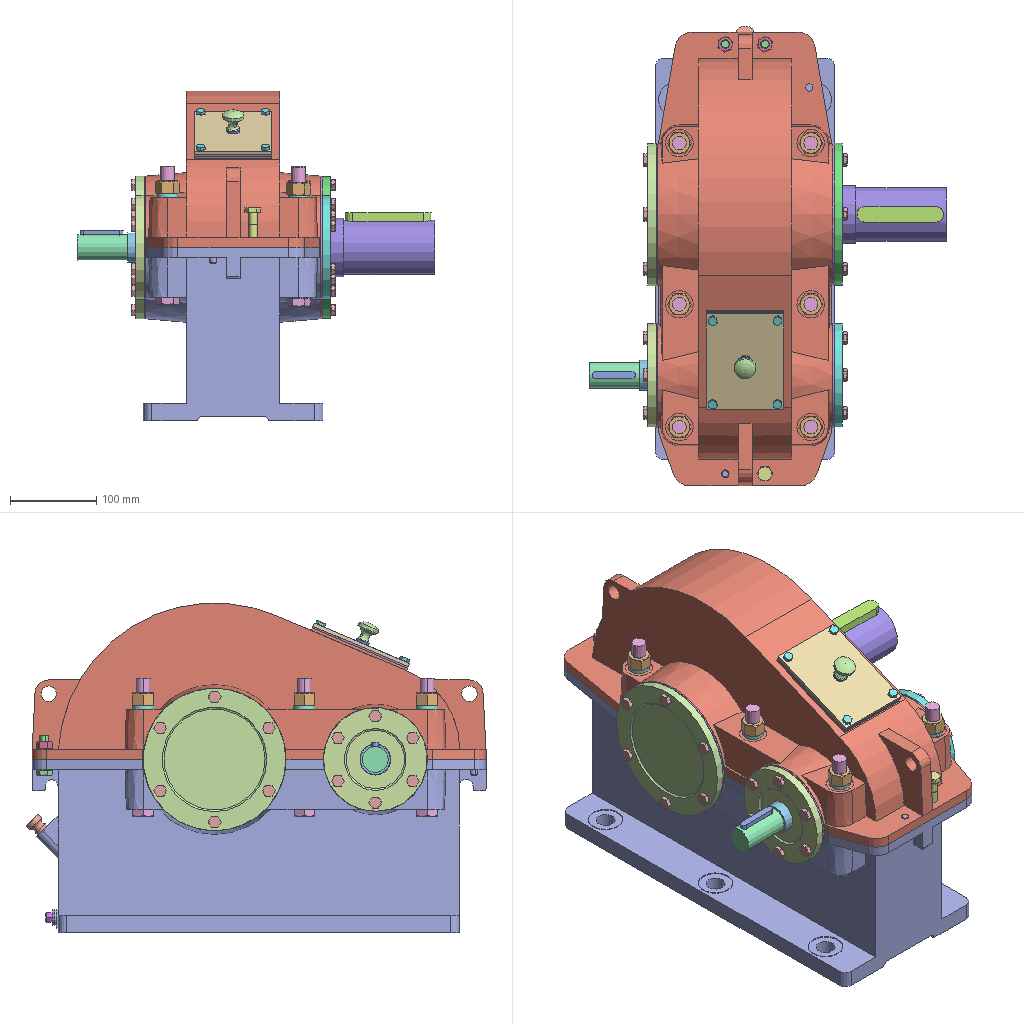Assembly | NX | 39 different items | 95 placed | box 413 x 532 x 381 mm
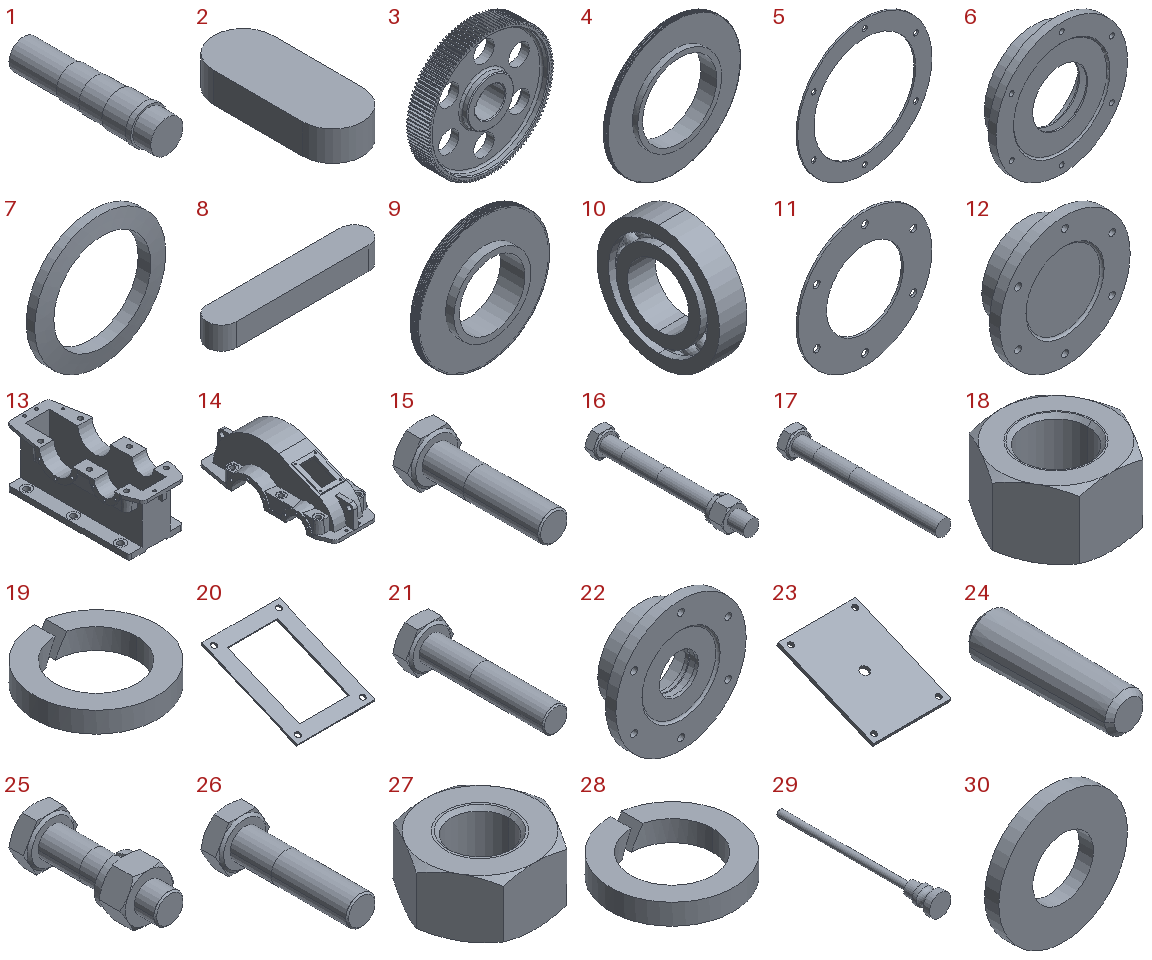Parts list (item | quantity | parent item | size | volume | features):
1 | x1 | - | 79 x 311 x 79 mm | 1137641 mm3 | features DATUM_CSYS 9, EXTRUDE 8, SKETCH 8, BLEND 2
2 | x1 | - | 20 x 50 x 10 mm | 9142 mm3 | features DATUM_CSYS 2, EXTRUDE 1, SKETCH 1
3 | x1 | - | 322.473 x 55 x 322.494 mm | 1796167 mm3 | features BREP 127, META 127, DATUM_CSYS 10, SKETCH 9, EXTRACT_DATUM_AXIS 8, HOLE PACKAGE 7, SIMPLE HOLE 7, EXTRACT_FACE 6, Instance Feature 6, EXTRUDE 3, EXTRACT_DATUM_PLANE 2, BLEND 1, CHAMFER 1, CYLINDER 1, FSET 1, Mirror Feature 1, Pattern Feature 1
4 | x2 | - | 125 x 15 x 125 mm | 52069 mm3 | features DATUM_CSYS 4, SKETCH 3, EXTRUDE 2, HOLE PACKAGE 1, SIMPLE HOLE 1, SWP104 1
5 | x2 | - | 165 x 2 x 165 mm | 17882 mm3 | features DATUM_CSYS 12, SKETCH 11, HOLE PACKAGE 9, SIMPLE HOLE 9, EXTRACT_DATUM_AXIS 6, EXTRACT_FACE 6, Instance Feature 5, EXTRUDE 4, BLEND 2, DELETE FACE 1, OFFSET_REGION 1, Pattern Feature 1, SWP104 1
6 | x1 | - | 165 x 34.6 x 165 mm | 207010 mm3 | features DATUM_CSYS 10, HOLE PACKAGE 9, SIMPLE HOLE 9, SKETCH 9, EXTRACT_DATUM_AXIS 6, EXTRACT_FACE 6, Instance Feature 5, BLEND 2, EXTRUDE 2, Pattern Feature 1, SWP104 1
7 | x1 | - | 93.171 x 8.968 x 93.171 mm | 22814 mm3 | features DATUM_CSYS 3, SKETCH 2, EXTRUDE 1, SWP104 1
8 | x1 | - | 100 x 18 x 14 mm | 24227 mm3 | features DATUM_CSYS 2, BLEND 1, EXTRUDE 1, SKETCH 1
9 | x2 | - | 80 x 15 x 80 mm | 23126 mm3 | features DATUM_CSYS 5, SKETCH 4, EXTRUDE 3, SWP104 1
10 | x2 | - | 18 x 80 x 80 mm | 52959 mm3 | features BREP 17
11 | x2 | - | 120 x 2 x 120 mm | 14781 mm3 | features DATUM_CSYS 12, SKETCH 11, HOLE PACKAGE 9, SIMPLE HOLE 9, EXTRACT_DATUM_AXIS 6, EXTRACT_FACE 6, Instance Feature 5, EXTRUDE 4, BLEND 2, DELETE FACE 1, Pattern Feature 1, REPLACE_FACE 1, SWP104 1
12 | x1 | - | 120 x 36.6 x 120 mm | 144277 mm3 | features DATUM_CSYS 9, HOLE PACKAGE 9, SIMPLE HOLE 9, SKETCH 8, EXTRACT_DATUM_AXIS 6, EXTRACT_FACE 6, Instance Feature 5, BLEND 2, EXTRUDE 2, DELETE FACE 1, Pattern Feature 1
13 | x1 | - | 208 x 525 x 200.222 mm | 4335166 mm3 | features SIMPLE HOLE 56, DATUM_CSYS 27, HOLE PACKAGE 26, SKETCH 26, EXTRUDE 18, EXTRACT_FACE 16, EXTRACT_DATUM_AXIS 10, BLEND 8, CBORE_HOLE 7, EXTRACT_DATUM_PLANE 6, FSET 6, Instance Feature 5, Mirror Feature 5, DRAFT 4, EXTRACT_STRING 2
14 | x1 | - | 202 x 525 x 181 mm | 2847836 mm3 | features SIMPLE HOLE 56, DATUM_CSYS 27, HOLE PACKAGE 26, SKETCH 26, EXTRUDE 18, EXTRACT_FACE 16, EXTRACT_DATUM_AXIS 10, BLEND 8, CBORE_HOLE 7, EXTRACT_DATUM_PLANE 6, FSET 6, Instance Feature 5, Mirror Feature 5, DRAFT 4, EXTRACT_STRING 2
15 | x1 | - | 18.475 x 46.4 x 16 mm | 5258 mm3 | features BREP 2
16 | x6 | - | 27.713 x 160 x 24.4 mm | 46237 mm3 | features BREP 5, DELETE FACE 1, OFFSET_REGION 1
17 | x6 | in 16 | 27.713 x 160 x 24 mm | 38117 mm3 | features BREP 2, DELETE FACE 1, OFFSET_REGION 1
18 | x6 | in 16 | 27.713 x 24 x 14.8 mm | 7082 mm3 | features BREP 2
19 | x6 | in 16 | 24.4 x 24.4 x 4.1 mm | 1037 mm3 | features BREP 1
20 | x1 | - | 90 x 111.242 x 48.729 mm | 10934 mm3 | features SIMPLE HOLE 56, DATUM_CSYS 27, HOLE PACKAGE 26, SKETCH 26, EXTRUDE 18, EXTRACT_FACE 16, EXTRACT_DATUM_AXIS 10, BLEND 8, CBORE_HOLE 7, EXTRACT_DATUM_PLANE 6, FSET 6, Instance Feature 5, Mirror Feature 5, DRAFT 4, EXTRACT_STRING 2, OFFSET_REGION 1
21 | x4 | - | 11.547 x 34 x 10 mm | 1354 mm3 | features BREP 2
22 | x1 | - | 120 x 36.6 x 120 mm | 131277 mm3 | features DATUM_CSYS 10, HOLE PACKAGE 9, SIMPLE HOLE 9, SKETCH 9, EXTRACT_DATUM_AXIS 6, EXTRACT_FACE 6, Instance Feature 5, BLEND 2, EXTRUDE 2, Pattern Feature 1, SWP104 1
23 | x1 | - | 90 x 112.024 x 50.57 mm | 42433 mm3 | features SIMPLE HOLE 57, DATUM_CSYS 28, HOLE PACKAGE 27, SKETCH 27, EXTRUDE 18, EXTRACT_FACE 16, EXTRACT_DATUM_AXIS 10, BLEND 8, CBORE_HOLE 7, EXTRACT_DATUM_PLANE 6, FSET 6, Instance Feature 5, Mirror Feature 5, DRAFT 4, EXTRACT_STRING 2, DELETE FACE 1, OFFSET_REGION 1
24 | x1 | - | 8.911 x 30 x 8.911 mm | 1668 mm3 | features BREP 1
25 | x2 | - | 18.475 x 46.4 x 16 mm | 7344 mm3 | features BREP 5
26 | x2 | in 25 | 18.475 x 46.4 x 16 mm | 5258 mm3 | features BREP 2
27 | x2 | in 25 | 18.475 x 16 x 8.4 mm | 1823 mm3 | features BREP 2
28 | x2 | in 25 | 15.4 x 15.4 x 2.6 mm | 263.016 mm3 | features BREP 1
29 | x1 | - | 20 x 148 x 20 mm | 8375 mm3 | features DATUM_CSYS 6, SKETCH 5, EXTRUDE 4, SWP104 1
30 | x1 | - | 18 x 2 x 18 mm | 395.448 mm3 | features DATUM_CSYS 2, EXTRUDE 1, SKETCH 1
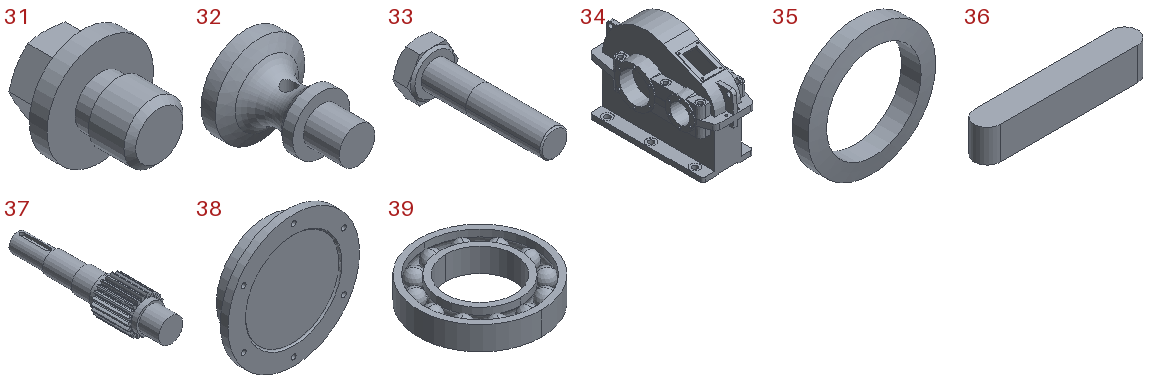31 | x1 | - | 18 x 20 x 18 mm | 2187 mm3 | features DATUM_CSYS 6, SKETCH 5, EXTRUDE 4, CHAMFER 1, SWP104 1
32 | x1 | - | 25 x 35 x 25 mm | 6314 mm3 | features DATUM_CSYS 5, SKETCH 4, EXTRUDE 3, SWP104 1
33 | x24 | - | 15.011 x 40.3 x 13 mm | 2901 mm3 | features BREP 2
34 | x1 | - | 208 x 525 x 381.222 mm | 7183001 mm3 | features SIMPLE HOLE 56, DATUM_CSYS 26, HOLE PACKAGE 26, SKETCH 25, EXTRUDE 17, EXTRACT_FACE 16, EXTRACT_DATUM_AXIS 10, BLEND 8, CBORE_HOLE 7, EXTRACT_DATUM_PLANE 6, FSET 6, Instance Feature 5, Mirror Feature 5, DRAFT 4, EXTRACT_STRING 2
35 | x1 | - | 48.653 x 7.48 x 48.653 mm | 5606 mm3 | features DATUM_CSYS 3, SKETCH 2, EXTRUDE 1, SWP104 1
36 | x1 | - | 50 x 8 x 10 mm | 3863 mm3 | features DATUM_CSYS 2, BLEND 1, EXTRUDE 1, SKETCH 1
37 | x1 | - | 60 x 252 x 59.615 mm | 341814 mm3 | features BREP 22, META 22, DATUM_CSYS 8, EXTRUDE 7, SKETCH 7, EXTRACT_DATUM_AXIS 2, EXTRACT_DATUM_PLANE 2, BLEND 1, CYLINDER 1, FSET 1, Instance Feature 1, Mirror Feature 1
38 | x1 | - | 165 x 34.6 x 165 mm | 267748 mm3 | features DATUM_CSYS 9, HOLE PACKAGE 9, SIMPLE HOLE 9, SKETCH 8, EXTRACT_DATUM_AXIS 6, EXTRACT_FACE 6, Instance Feature 5, BLEND 2, EXTRUDE 2, DELETE FACE 1, Pattern Feature 1
39 | x2 | - | 125 x 125 x 24 mm | 122130 mm3 | features BREP 14
Mates (type | each side: item.copy, entity, surface, feature):
In the top assembly
Fix | 13.1 component
Touch | 37.1 face cylinder Extrude(50) | 13.1 face cylinder Ø80 Hole(32)
Distance | 37.1 face plane Cylinder(1) | 13.1 face plane Extrude(43)
Touch | 1.1 face cylinder Extrude(6) | 13.1 face cylinder Ø125 Hole(33)
Distance | 1.1 face plane Extrude(2) | 13.1 face plane Extrude(43)
Parallel | 1.1 face plane Extrude(9) | 13.1 face plane Extrude(4)
Touch | 2.1 face cylinder Extrude(1) | 1.1 face cylinder Edge Blend(10) | 2 times
Touch | 2.1 face plane Extrude(1) | 1.1 face plane Extrude(9)
Touch | 3.1 face cylinder Ø75 Hole(257) | 1.1 face cylinder Extrude(4)
Touch | 3.1 face plane Cylinder(1) | 1.1 face plane Extrude(2)
Parallel | 3.1 face plane Extrude(263) | 1.1 face plane Extrude(7)
Touch | 11.1 face cylinder Pattern Feature [Circular] (10) / Instance[3][0] | 13.1 face cylinder Mirror Feature(41)
Touch | 11.1 face plane Extrude(1) | 13.1 face plane Mirror Feature(10)
Touch | 11.1 face cylinder Pattern Feature [Circular] (10) / Instance[3][0] | 13.1 face cylinder Ø10 Hole(40)
Touch | 11.1 face plane Extrude(13) | 13.1 face plane Extrude(3)
Touch | 22.1 face cylinder Revolve(7) | 37.1 face cylinder Extrude(51)
Touch | 22.1 face cylinder Pattern Feature [Circular] (10) / Instance[1][0] | 11.1 face cylinder Pattern Feature [Circular] (10) / Instance[3][0]
Touch | 22.1 face plane Extrude(1) | 11.1 face plane Extrude(13)
Touch | 9.1 face cylinder Extrude(4) | 37.1 face cylinder Extrude(50)
Touch | 9.1 face plane Extrude(1) | 37.1 face plane Mirror Feature(48)
Touch | 10.1 face cylinder Body(1) | 37.1 face cylinder Extrude(51)
Touch | 10.1 face plane Body(2) | 9.1 face plane Extrude(1)
Touch | 9.1 face cylinder Extrude(4) | 37.1 face cylinder Extrude(49)
Touch | 9.1 face plane Extrude(1) | 37.1 face plane Extrude(47)
Touch | 10.1 face cylinder Body(1) | 37.1 face cylinder Extrude(49)
Touch | 10.1 face plane Body(1) | 9.1 face plane Extrude(1)
Touch | 12.1 face cylinder Extrude(1) | 10.1 face cylinder Body(2)
Touch | 12.1 face cylinder Pattern Feature [Circular] (10) / Instance[3][0] | 11.1 face cylinder Pattern Feature [Circular] (10) / Instance[3][0]
Touch | 12.1 face plane Extrude(1) | 11.1 face plane Extrude(1)
Touch | 5.1 face cylinder Pattern Feature [Circular] (10) / Instance[3][0] | 13.1 face cylinder Mirror Feature(41)
Touch | 5.1 face plane Extrude(1) | 13.1 face plane Mirror Feature(10)
Touch | 5.1 face cylinder Extrude(14) | 1.1 face cylinder Extrude(4)
Touch | 5.1 face cylinder Pattern Feature [Circular] (10) / Instance[3][0] | 13.1 face cylinder Ø10 Hole(40)
Touch | 5.1 face plane Extrude(13) | 13.1 face plane Extrude(3)
Touch | 38.1 face cylinder Extrude(1) | 13.1 face cylinder Ø125 Hole(33)
Touch | 38.1 face cylinder Pattern Feature [Circular] (10) / Instance[1][0] | 5.1 face cylinder Pattern Feature [Circular] (10) / Instance[3][0]
Touch | 38.1 face plane Extrude(1) | 5.1 face plane Extrude(13)
Touch | 4.1 face cylinder Ø70 Hole(4) | 1.1 face cylinder Extrude(1)
Touch | 4.1 face plane Extrude(1) | 1.1 face plane Extrude(2)
Touch | 39.1 face cylinder Body(1) | 4.1 face cylinder Extrude(1)
Touch | 39.1 face plane Body(2) | 4.1 face plane Extrude(1)
Touch | 4.1 face cylinder Ø70 Hole(4) | 1.1 face cylinder Extrude(4)
Touch | 4.1 face plane Extrude(1) | 3.1 face plane Cylinder(1)
Touch | 39.1 face cylinder Body(1) | 1.1 face cylinder Extrude(4)
Touch | 6.1 face cylinder Ø69 Hole(4) | 1.1 face cylinder Extrude(6)
Touch | 6.1 face cylinder Pattern Feature [Circular] (10) / Instance[5][0] | 13.1 face cylinder Ø10 Hole(40)
Touch | 6.1 face plane Extrude(1) | 5.1 face plane Extrude(1)
Touch | 14.1 face cylinder Ø80 Hole(32) | 12.1 face surfaceofrevolution Edge Blend(6)
Touch | 14.1 face cylinder Ø125 Hole(33) | 1.1 face cylinder Extrude(6)
Touch | 14.1 face plane Extrude(4) | 13.1 face plane Extrude(4)
Touch | 20.1 face plane Extrude(49) | 14.1 face plane Extrude(15)
Touch | 20.1 face plane Extrude(15) | 14.1 face plane Extrude(15) | 2 times
Touch | 23.1 face plane Extrude(49) | 20.1 face plane Extrude(15)
Touch | 23.1 face plane Extrude(15) | 14.1 face plane Extrude(15) | 2 times
Touch | 21.1 face cylinder Body(1) | 23.1 face cylinder Ø6 Hole(47) | 4 times
Touch | 21.1 face plane Body(1) | 23.1 face plane Extrude(15) | 4 times
Touch | 32.1 face plane Extrude(2) | 23.1 face plane Extrude(15)
Touch | 32.1 face cylinder Extrude(2) | 23.1 face cylinder Ø10 Hole(51)
Touch | 29.1 face plane Extrude(2) | 13.1 face plane Ø12 Counterbored Hole(45)
Touch | 29.1 face cylinder Extrude(5) | 13.1 face cylinder Edge Blend(21)
Touch | 30.1 face cylinder Extrude(1) | 31.1 face cylinder Extrude(1)
Touch | 30.1 face plane Extrude(1) | 31.1 face plane Extrude(3)
Touch | 31.1 face cylinder Extrude(1) | 13.1 face cylinder Ø10 Hole(44)
Touch | 30.1 face plane Extrude(1) | 13.1 face plane Extrude(22)
Touch | 15.1 face plane Body(1) | 13.1 face plane Ø10 Hole(36)
Touch | 15.1 face cylinder Body(1) | 14.1 face cylinder Ø10 Hole(36)
Touch | 26.1 face cylinder Body(1) | 14.1 face cylinder Ø11 Hole(34) | 2 times
Touch | 26.1 face plane Body(1) | 13.1 face plane Extrude(1) | 2 times
Touch | 24.1 face plane Body(1) | 14.1 face plane Extrude(1)
Touch | 24.1 face cone Body(1) | 14.1 face cylinder Ø9 Hole(35)
Parallel | 37.1 face plane Extrude(53) | 14.1 face plane Extrude(1)
Touch | 19.1 face plane Body(1) | 14.1 face plane Mirror Feature(31)
Touch | 17.1 face cylinder Body(1) | 14.1 face cylinder Mirror Feature(31) | 2 times
Touch | 17.1 face plane Body(1) | 13.1 face plane Mirror Feature(31) | 2 times
Touch | 17.1 face cylinder Body(1) | 13.1 face cylinder Mirror Feature(31)
Touch | 17.1 face plane Body(1) | 13.1 face plane Mirror Feature(29) | 3 times
Touch | 17.1 face cylinder Body(1) | 13.1 face cone Mirror Feature(11)
Touch | 17.1 face cylinder Body(1) | 13.1 face cylinder Ø17 Hole(24) | 2 times
Touch | 33.1 face plane Body(1) | 12.1 face plane Extrude(1)
Touch | 33.1 face cylinder Body(1) | 12.1 face cylinder Ø6 Hole(9)
Fix | assembly component | 4 times
Bond | 33.1 component | assembly component | 24 times
CircularPattern | assembly axis | assembly csys | assembly csys | assembly csys | assembly csys | assembly csys | assembly csys | 4 times
Touch | 33.1 face cylinder Body(1) | 6.1 face cylinder Pattern Feature [Circular] (10) / Instance[2][0]
Touch | 33.1 face plane Body(1) | 6.1 face plane Extrude(1)
Touch | 33.1 face cylinder Body(1) | 38.1 face cylinder Pattern Feature [Circular] (10) / Instance[4][0]
Touch | 33.1 face plane Body(1) | 38.1 face plane Extrude(1)
Touch | 33.1 face cylinder Body(1) | 22.1 face cylinder Pattern Feature [Circular] (10) / Instance[4][0]
Touch | 33.1 face plane Body(1) | 22.1 face plane Extrude(1)
Touch | 8.1 face plane Extrude(1) | 1.1 face plane Extrude(7)
Touch | 8.1 face cylinder Edge Blend(2) | 1.1 face cylinder Edge Blend(8)
Touch | 36.1 face plane Extrude(1) | 37.1 face plane Extrude(53)
Touch | 36.1 face cylinder Edge Blend(2) | 37.1 face cylinder Edge Blend(54)
In subassembly 16
Touch | 19.1 | 17.1
Distance | 19.1 | 17.1
Touch | 18.1 | 17.1
Touch | 18.1 | 19.1
In subassembly 25
Touch | 28.1 | 26.1
Distance | 28.1 | 26.1
Touch | 27.1 | 26.1
Touch | 27.1 | 28.1